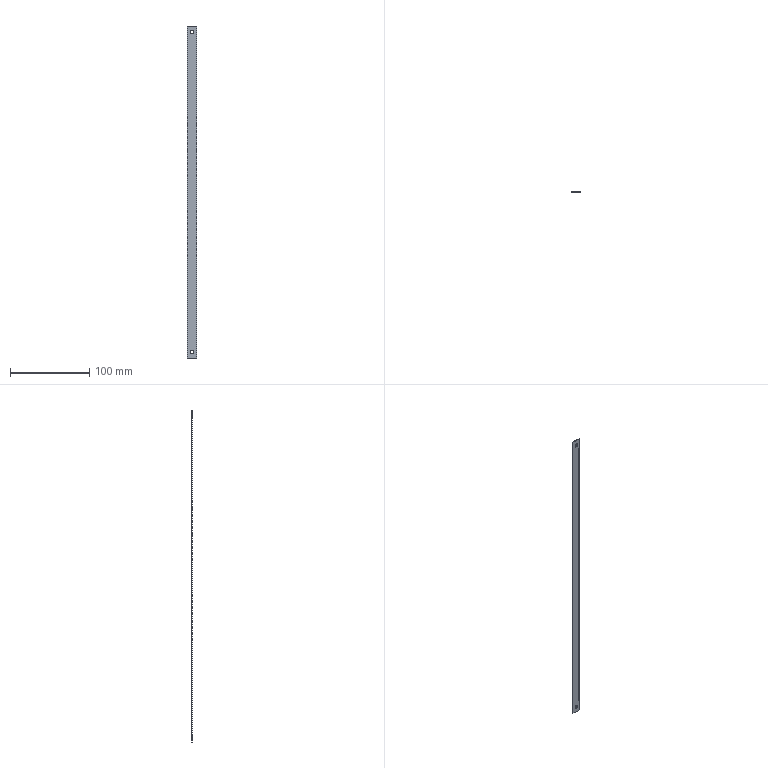Part | STEP file | Scale ruler | 1 solid | 1574 faces | box 12 x 1 x 420 mm | volume 4971 mm3 | plane 1570 | cylinder 4 | commonest cylinder face diameters 4.5 x4